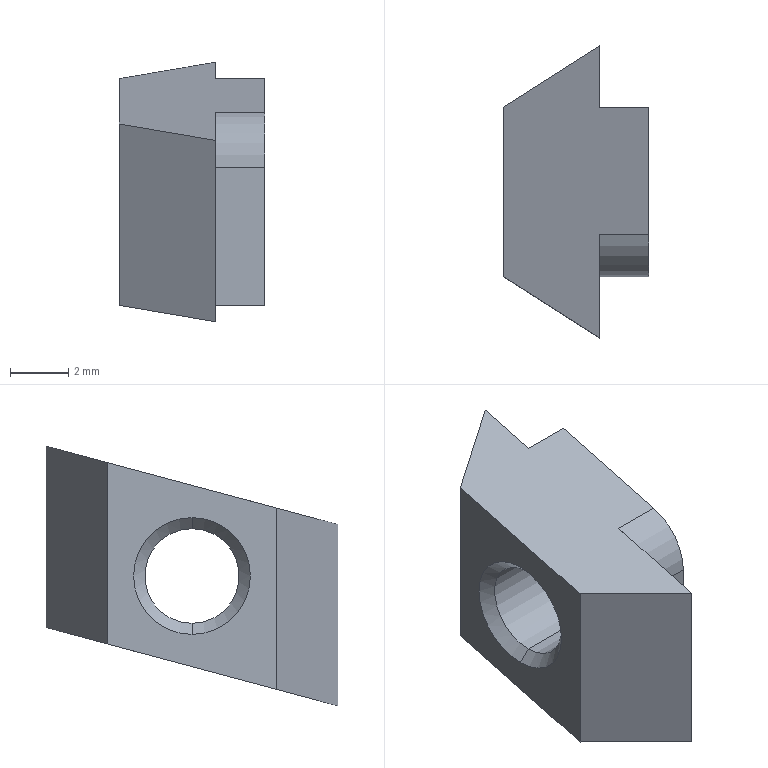Part | STEP file | 0245_026_HNTFSN5-4 | 1 solid | 18 faces | box 5 x 10 x 8.891 mm | volume 178.899 mm3 | plane 10 | cone 4 | cylinder 4 | commonest cylinder face diameters 3.242 x2 3.867 x2
STEP:
#1=CARTESIAN_POINT('',(0.,0.,0.));
#2=DIRECTION('',(0.,0.,1.));
#3=DIRECTION('',(1.,0.,0.));
#4=AXIS2_PLACEMENT_3D('',#1,#2,#3);
#5=CARTESIAN_POINT('',(-4.621,0.,1.621));
#6=VERTEX_POINT('',#5);
#7=CARTESIAN_POINT('',(-5.,0.,2.));
#8=VERTEX_POINT('',#7);
#9=CARTESIAN_POINT('',(-5.,0.,2.));
#10=DIRECTION('',(-0.7071,0.,0.7071));
#11=VECTOR('',#10,1.);
#12=LINE('',#9,#11);
#13=CARTESIAN_POINT('',(-5.,0.,0.));
#14=DIRECTION('',(-1.,0.,0.));
#15=DIRECTION('',(0.,0.,1.));
#16=AXIS2_PLACEMENT_3D('',#13,#14,#15);
#17=CONICAL_SURFACE('',#16,2.,0.7854);
#18=CARTESIAN_POINT('',(6.283,0.));
#19=DIRECTION('',(0.,1.));
#20=VECTOR('',#19,1.);
#21=LINE('',#18,#20);
#22=(GEOMETRIC_REPRESENTATION_CONTEXT(2)PARAMETRIC_REPRESENTATION_CONTEXT()REPRESENTATION_CONTEXT('',''));
#23=DEFINITIONAL_REPRESENTATION('',(#21),#22);
#24=PCURVE('',#17,#23);
#25=CARTESIAN_POINT('',(-5.,0.,0.));
#26=DIRECTION('',(-1.,0.,0.));
#27=DIRECTION('',(0.,0.,1.));
#28=AXIS2_PLACEMENT_3D('',#25,#26,#27);
#29=CONICAL_SURFACE('',#28,2.,0.7854);
#30=CARTESIAN_POINT('',(0.,0.));
#31=DIRECTION('',(0.,1.));
#32=VECTOR('',#31,1.);
#33=LINE('',#30,#32);
#34=(GEOMETRIC_REPRESENTATION_CONTEXT(2)PARAMETRIC_REPRESENTATION_CONTEXT()REPRESENTATION_CONTEXT('',''));
#35=DEFINITIONAL_REPRESENTATION('',(#33),#34);
#36=PCURVE('',#29,#35);
#37=SURFACE_CURVE('',#12,(#24,#36),.PCURVE_S1.);
#38=EDGE_CURVE('',#6,#8,#37,.T.);
#39=ORIENTED_EDGE('',*,*,#38,.T.);
#40=CARTESIAN_POINT('',(-5.,0.,-2.));
#41=VERTEX_POINT('',#40);
#42=CARTESIAN_POINT('',(-5.,0.,0.));
#43=DIRECTION('',(-1.,0.,0.));
#44=DIRECTION('',(0.,0.,1.));
#45=AXIS2_PLACEMENT_3D('',#42,#43,#44);
#46=CIRCLE('',#45,2.);
#47=CARTESIAN_POINT('',(0.,0.));
#48=DIRECTION('',(1.,0.));
#49=VECTOR('',#48,1.);
#50=LINE('',#47,#49);
#51=(GEOMETRIC_REPRESENTATION_CONTEXT(2)PARAMETRIC_REPRESENTATION_CONTEXT()REPRESENTATION_CONTEXT('',''));
#52=DEFINITIONAL_REPRESENTATION('',(#50),#51);
#53=PCURVE('',#17,#52);
#54=CARTESIAN_POINT('',(-5.,0.,0.));
#55=DIRECTION('',(1.,0.,0.));
#56=DIRECTION('',(0.,0.,-1.));
#57=AXIS2_PLACEMENT_3D('',#54,#55,#56);
#58=PLANE('',#57);
#59=CARTESIAN_POINT('',(-2.,0.));
#60=CARTESIAN_POINT('',(-2.,3.464));
#61=CARTESIAN_POINT('',(1.,1.732));
#62=CARTESIAN_POINT('',(4.,0.));
#63=CARTESIAN_POINT('',(1.,-1.732));
#64=CARTESIAN_POINT('',(-2.,-3.464));
#65=CARTESIAN_POINT('',(-2.,0.));
#66=(BOUNDED_CURVE()B_SPLINE_CURVE(2,(#59,#60,#61,#62,#63,#64,#65),.UNSPECIFIED.,.T.,.F.)B_SPLINE_CURVE_WITH_KNOTS((1,2,2,2,2,1),(-2.094,0.,2.094,4.189,6.283,8.378),.UNSPECIFIED.)CURVE()GEOMETRIC_REPRESENTATION_ITEM()RATIONAL_B_SPLINE_CURVE((1.,0.5,1.,0.5,1.,0.5,1.))REPRESENTATION_ITEM(''));
#67=(GEOMETRIC_REPRESENTATION_CONTEXT(2)PARAMETRIC_REPRESENTATION_CONTEXT()REPRESENTATION_CONTEXT('',''));
#68=DEFINITIONAL_REPRESENTATION('',(#66),#67);
#69=PCURVE('',#58,#68);
#70=SURFACE_CURVE('',#46,(#53,#69),.PCURVE_S1.);
#71=EDGE_CURVE('',#41,#8,#70,.T.);
#72=ORIENTED_EDGE('',*,*,#71,.F.);
#73=CARTESIAN_POINT('',(-4.621,0.,-1.621));
#74=VERTEX_POINT('',#73);
#75=CARTESIAN_POINT('',(-5.,0.,-2.));
#76=DIRECTION('',(-0.7071,0.,-0.7071));
#77=VECTOR('',#76,1.);
#78=LINE('',#75,#77);
#79=CARTESIAN_POINT('',(3.142,0.));
#80=DIRECTION('',(0.,1.));
#81=VECTOR('',#80,1.);
#82=LINE('',#79,#81);
#83=(GEOMETRIC_REPRESENTATION_CONTEXT(2)PARAMETRIC_REPRESENTATION_CONTEXT()REPRESENTATION_CONTEXT('',''));
#84=DEFINITIONAL_REPRESENTATION('',(#82),#83);
#85=PCURVE('',#17,#84);
#86=CARTESIAN_POINT('',(3.142,0.));
#87=DIRECTION('',(0.,1.));
#88=VECTOR('',#87,1.);
#89=LINE('',#86,#88);
#90=(GEOMETRIC_REPRESENTATION_CONTEXT(2)PARAMETRIC_REPRESENTATION_CONTEXT()REPRESENTATION_CONTEXT('',''));
#91=DEFINITIONAL_REPRESENTATION('',(#89),#90);
#92=PCURVE('',#29,#91);
#93=SURFACE_CURVE('',#78,(#85,#92),.PCURVE_S1.);
#94=EDGE_CURVE('',#74,#41,#93,.T.);
#95=ORIENTED_EDGE('',*,*,#94,.F.);
#96=CARTESIAN_POINT('',(-4.621,0.,0.));
#97=DIRECTION('',(-1.,0.,0.));
#98=DIRECTION('',(0.,1.,0.));
#99=AXIS2_PLACEMENT_3D('',#96,#97,#98);
#100=CIRCLE('',#99,1.621);
#101=CARTESIAN_POINT('',(1.571,-0.379));
#102=DIRECTION('',(1.,0.));
#103=VECTOR('',#102,1.);
#104=LINE('',#101,#103);
#105=(GEOMETRIC_REPRESENTATION_CONTEXT(2)PARAMETRIC_REPRESENTATION_CONTEXT()REPRESENTATION_CONTEXT('',''));
#106=DEFINITIONAL_REPRESENTATION('',(#104),#105);
#107=PCURVE('',#17,#106);
#108=CARTESIAN_POINT('',(-2.5,0.,0.));
#109=DIRECTION('',(1.,0.,0.));
#110=DIRECTION('',(0.,0.,-1.));
#111=AXIS2_PLACEMENT_3D('',#108,#109,#110);
#112=CYLINDRICAL_SURFACE('',#111,1.621);
#113=CARTESIAN_POINT('',(7.854,-2.121));
#114=DIRECTION('',(-1.,0.));
#115=VECTOR('',#114,1.);
#116=LINE('',#113,#115);
#117=(GEOMETRIC_REPRESENTATION_CONTEXT(2)PARAMETRIC_REPRESENTATION_CONTEXT()REPRESENTATION_CONTEXT('',''));
#118=DEFINITIONAL_REPRESENTATION('',(#116),#117);
#119=PCURVE('',#112,#118);
#120=SURFACE_CURVE('',#100,(#107,#119),.PCURVE_S1.);
#121=EDGE_CURVE('',#74,#6,#120,.T.);
#122=ORIENTED_EDGE('',*,*,#121,.T.);
#123=EDGE_LOOP('',(#39,#72,#95,#122));
#124=FACE_BOUND('',#123,.F.);
#125=ADVANCED_FACE('',(#124),#17,.F.);
#126=CARTESIAN_POINT('',(-0.379,0.,-1.621));
#127=VERTEX_POINT('',#126);
#128=CARTESIAN_POINT('',(0.,0.,-2.));
#129=VERTEX_POINT('',#128);
#130=CARTESIAN_POINT('',(0.,0.,-2.));
#131=DIRECTION('',(0.7071,0.,-0.7071));
#132=VECTOR('',#131,1.);
#133=LINE('',#130,#132);
#134=CARTESIAN_POINT('',(0.,0.,0.));
#135=DIRECTION('',(1.,0.,0.));
#136=DIRECTION('',(0.,0.,-1.));
#137=AXIS2_PLACEMENT_3D('',#134,#135,#136);
#138=CONICAL_SURFACE('',#137,2.,0.7854);
#139=CARTESIAN_POINT('',(6.283,0.));
#140=DIRECTION('',(0.,1.));
#141=VECTOR('',#140,1.);
#142=LINE('',#139,#141);
#143=(GEOMETRIC_REPRESENTATION_CONTEXT(2)PARAMETRIC_REPRESENTATION_CONTEXT()REPRESENTATION_CONTEXT('',''));
#144=DEFINITIONAL_REPRESENTATION('',(#142),#143);
#145=PCURVE('',#138,#144);
#146=CARTESIAN_POINT('',(0.,0.,0.));
#147=DIRECTION('',(1.,0.,0.));
#148=DIRECTION('',(0.,0.,-1.));
#149=AXIS2_PLACEMENT_3D('',#146,#147,#148);
#150=CONICAL_SURFACE('',#149,2.,0.7854);
#151=CARTESIAN_POINT('',(0.,0.));
#152=DIRECTION('',(0.,1.));
#153=VECTOR('',#152,1.);
#154=LINE('',#151,#153);
#155=(GEOMETRIC_REPRESENTATION_CONTEXT(2)PARAMETRIC_REPRESENTATION_CONTEXT()REPRESENTATION_CONTEXT('',''));
#156=DEFINITIONAL_REPRESENTATION('',(#154),#155);
#157=PCURVE('',#150,#156);
#158=SURFACE_CURVE('',#133,(#145,#157),.PCURVE_S1.);
#159=EDGE_CURVE('',#127,#129,#158,.T.);
#160=ORIENTED_EDGE('',*,*,#159,.T.);
#161=CARTESIAN_POINT('',(0.,0.,2.));
#162=VERTEX_POINT('',#161);
#163=CARTESIAN_POINT('',(0.,0.,0.));
#164=DIRECTION('',(-1.,0.,0.));
#165=DIRECTION('',(0.,0.,-1.));
#166=AXIS2_PLACEMENT_3D('',#163,#164,#165);
#167=CIRCLE('',#166,2.);
#168=CARTESIAN_POINT('',(6.283,0.));
#169=DIRECTION('',(-1.,0.));
#170=VECTOR('',#169,1.);
#171=LINE('',#168,#170);
#172=(GEOMETRIC_REPRESENTATION_CONTEXT(2)PARAMETRIC_REPRESENTATION_CONTEXT()REPRESENTATION_CONTEXT('',''));
#173=DEFINITIONAL_REPRESENTATION('',(#171),#172);
#174=PCURVE('',#138,#173);
#175=CARTESIAN_POINT('',(0.,0.,0.));
#176=DIRECTION('',(1.,0.,0.));
#177=DIRECTION('',(0.,0.,-1.));
#178=AXIS2_PLACEMENT_3D('',#175,#176,#177);
#179=PLANE('',#178);
#180=CARTESIAN_POINT('',(2.,0.));
#181=CARTESIAN_POINT('',(2.,-3.464));
#182=CARTESIAN_POINT('',(-1.,-1.732));
#183=CARTESIAN_POINT('',(-4.,0.));
#184=CARTESIAN_POINT('',(-1.,1.732));
#185=CARTESIAN_POINT('',(2.,3.464));
#186=CARTESIAN_POINT('',(2.,0.));
#187=(BOUNDED_CURVE()B_SPLINE_CURVE(2,(#180,#181,#182,#183,#184,#185,#186),.UNSPECIFIED.,.T.,.F.)B_SPLINE_CURVE_WITH_KNOTS((1,2,2,2,2,1),(-2.094,0.,2.094,4.189,6.283,8.378),.UNSPECIFIED.)CURVE()GEOMETRIC_REPRESENTATION_ITEM()RATIONAL_B_SPLINE_CURVE((1.,0.5,1.,0.5,1.,0.5,1.))REPRESENTATION_ITEM(''));
#188=(GEOMETRIC_REPRESENTATION_CONTEXT(2)PARAMETRIC_REPRESENTATION_CONTEXT()REPRESENTATION_CONTEXT('',''));
#189=DEFINITIONAL_REPRESENTATION('',(#187),#188);
#190=PCURVE('',#179,#189);
#191=SURFACE_CURVE('',#167,(#174,#190),.PCURVE_S1.);
#192=EDGE_CURVE('',#129,#162,#191,.T.);
#193=ORIENTED_EDGE('',*,*,#192,.T.);
#194=CARTESIAN_POINT('',(-0.379,0.,1.621));
#195=VERTEX_POINT('',#194);
#196=CARTESIAN_POINT('',(0.,0.,2.));
#197=DIRECTION('',(0.7071,0.,0.7071));
#198=VECTOR('',#197,1.);
#199=LINE('',#196,#198);
#200=CARTESIAN_POINT('',(3.142,0.));
#201=DIRECTION('',(0.,1.));
#202=VECTOR('',#201,1.);
#203=LINE('',#200,#202);
#204=(GEOMETRIC_REPRESENTATION_CONTEXT(2)PARAMETRIC_REPRESENTATION_CONTEXT()REPRESENTATION_CONTEXT('',''));
#205=DEFINITIONAL_REPRESENTATION('',(#203),#204);
#206=PCURVE('',#138,#205);
#207=CARTESIAN_POINT('',(3.142,0.));
#208=DIRECTION('',(0.,1.));
#209=VECTOR('',#208,1.);
#210=LINE('',#207,#209);
#211=(GEOMETRIC_REPRESENTATION_CONTEXT(2)PARAMETRIC_REPRESENTATION_CONTEXT()REPRESENTATION_CONTEXT('',''));
#212=DEFINITIONAL_REPRESENTATION('',(#210),#211);
#213=PCURVE('',#150,#212);
#214=SURFACE_CURVE('',#199,(#206,#213),.PCURVE_S1.);
#215=EDGE_CURVE('',#195,#162,#214,.T.);
#216=ORIENTED_EDGE('',*,*,#215,.F.);
#217=CARTESIAN_POINT('',(-0.379,0.,0.));
#218=DIRECTION('',(1.,0.,0.));
#219=DIRECTION('',(0.,1.,0.));
#220=AXIS2_PLACEMENT_3D('',#217,#218,#219);
#221=CIRCLE('',#220,1.621);
#222=CARTESIAN_POINT('',(1.571,-0.379));
#223=DIRECTION('',(1.,0.));
#224=VECTOR('',#223,1.);
#225=LINE('',#222,#224);
#226=(GEOMETRIC_REPRESENTATION_CONTEXT(2)PARAMETRIC_REPRESENTATION_CONTEXT()REPRESENTATION_CONTEXT('',''));
#227=DEFINITIONAL_REPRESENTATION('',(#225),#226);
#228=PCURVE('',#138,#227);
#229=CARTESIAN_POINT('',(1.571,2.121));
#230=DIRECTION('',(1.,0.));
#231=VECTOR('',#230,1.);
#232=LINE('',#229,#231);
#233=(GEOMETRIC_REPRESENTATION_CONTEXT(2)PARAMETRIC_REPRESENTATION_CONTEXT()REPRESENTATION_CONTEXT('',''));
#234=DEFINITIONAL_REPRESENTATION('',(#232),#233);
#235=PCURVE('',#112,#234);
#236=SURFACE_CURVE('',#221,(#228,#235),.PCURVE_S1.);
#237=EDGE_CURVE('',#195,#127,#236,.T.);
#238=ORIENTED_EDGE('',*,*,#237,.T.);
#239=EDGE_LOOP('',(#160,#193,#216,#238));
#240=FACE_BOUND('',#239,.F.);
#241=ADVANCED_FACE('',(#240),#138,.F.);
#242=CARTESIAN_POINT('',(-2.5,0.,-1.621));
#243=DIRECTION('',(1.,0.,0.));
#244=VECTOR('',#243,1.);
#245=LINE('',#242,#244);
#246=CARTESIAN_POINT('',(6.283,0.));
#247=DIRECTION('',(0.,1.));
#248=VECTOR('',#247,1.);
#249=LINE('',#246,#248);
#250=(GEOMETRIC_REPRESENTATION_CONTEXT(2)PARAMETRIC_REPRESENTATION_CONTEXT()REPRESENTATION_CONTEXT('',''));
#251=DEFINITIONAL_REPRESENTATION('',(#249),#250);
#252=PCURVE('',#112,#251);
#253=CARTESIAN_POINT('',(-2.5,0.,0.));
#254=DIRECTION('',(1.,0.,0.));
#255=DIRECTION('',(0.,0.,-1.));
#256=AXIS2_PLACEMENT_3D('',#253,#254,#255);
#257=CYLINDRICAL_SURFACE('',#256,1.621);
#258=CARTESIAN_POINT('',(0.,0.));
#259=DIRECTION('',(0.,1.));
#260=VECTOR('',#259,1.);
#261=LINE('',#258,#260);
#262=(GEOMETRIC_REPRESENTATION_CONTEXT(2)PARAMETRIC_REPRESENTATION_CONTEXT()REPRESENTATION_CONTEXT('',''));
#263=DEFINITIONAL_REPRESENTATION('',(#261),#262);
#264=PCURVE('',#257,#263);
#265=SURFACE_CURVE('',#245,(#252,#264),.PCURVE_S1.);
#266=EDGE_CURVE('',#74,#127,#265,.T.);
#267=ORIENTED_EDGE('',*,*,#266,.T.);
#268=ORIENTED_EDGE('',*,*,#237,.F.);
#269=CARTESIAN_POINT('',(-2.5,0.,1.621));
#270=DIRECTION('',(1.,0.,0.));
#271=VECTOR('',#270,1.);
#272=LINE('',#269,#271);
#273=CARTESIAN_POINT('',(3.142,0.));
#274=DIRECTION('',(0.,1.));
#275=VECTOR('',#274,1.);
#276=LINE('',#273,#275);
#277=(GEOMETRIC_REPRESENTATION_CONTEXT(2)PARAMETRIC_REPRESENTATION_CONTEXT()REPRESENTATION_CONTEXT('',''));
#278=DEFINITIONAL_REPRESENTATION('',(#276),#277);
#279=PCURVE('',#112,#278);
#280=CARTESIAN_POINT('',(3.142,0.));
#281=DIRECTION('',(0.,1.));
#282=VECTOR('',#281,1.);
#283=LINE('',#280,#282);
#284=(GEOMETRIC_REPRESENTATION_CONTEXT(2)PARAMETRIC_REPRESENTATION_CONTEXT()REPRESENTATION_CONTEXT('',''));
#285=DEFINITIONAL_REPRESENTATION('',(#283),#284);
#286=PCURVE('',#257,#285);
#287=SURFACE_CURVE('',#272,(#279,#286),.PCURVE_S1.);
#288=EDGE_CURVE('',#6,#195,#287,.T.);
#289=ORIENTED_EDGE('',*,*,#288,.F.);
#290=ORIENTED_EDGE('',*,*,#121,.F.);
#291=EDGE_LOOP('',(#267,#268,#289,#290));
#292=FACE_BOUND('',#291,.F.);
#293=ADVANCED_FACE('',(#292),#112,.F.);
#294=CARTESIAN_POINT('',(-5.,-2.9,-3.883));
#295=VERTEX_POINT('',#294);
#296=CARTESIAN_POINT('',(-5.,2.9,-2.329));
#297=VERTEX_POINT('',#296);
#298=CARTESIAN_POINT('',(-5.,-5.,-4.446));
#299=DIRECTION('',(0.,0.9659,0.2588));
#300=VECTOR('',#299,1.);
#301=LINE('',#298,#300);
#302=CARTESIAN_POINT('',(0.,-5.,-4.446));
#303=DIRECTION('',(0.,0.2588,-0.9659));
#304=DIRECTION('',(0.,0.9659,0.2588));
#305=AXIS2_PLACEMENT_3D('',#302,#303,#304);
#306=PLANE('',#305);
#307=CARTESIAN_POINT('',(0.,-5.));
#308=DIRECTION('',(1.,0.));
#309=VECTOR('',#308,1.);
#310=LINE('',#307,#309);
#311=(GEOMETRIC_REPRESENTATION_CONTEXT(2)PARAMETRIC_REPRESENTATION_CONTEXT()REPRESENTATION_CONTEXT('',''));
#312=DEFINITIONAL_REPRESENTATION('',(#310),#311);
#313=PCURVE('',#306,#312);
#314=CARTESIAN_POINT('',(4.446,-5.));
#315=DIRECTION('',(-0.2588,0.9659));
#316=VECTOR('',#315,1.);
#317=LINE('',#314,#316);
#318=(GEOMETRIC_REPRESENTATION_CONTEXT(2)PARAMETRIC_REPRESENTATION_CONTEXT()REPRESENTATION_CONTEXT('',''));
#319=DEFINITIONAL_REPRESENTATION('',(#317),#318);
#320=PCURVE('',#58,#319);
#321=SURFACE_CURVE('',#301,(#313,#320),.PCURVE_S1.);
#322=EDGE_CURVE('',#295,#297,#321,.T.);
#323=ORIENTED_EDGE('',*,*,#322,.T.);
#324=CARTESIAN_POINT('',(-1.7,5.,-1.766));
#325=VERTEX_POINT('',#324);
#326=CARTESIAN_POINT('',(-5.,2.9,-2.329));
#327=DIRECTION('',(0.8351,0.5314,0.1424));
#328=VECTOR('',#327,1.);
#329=LINE('',#326,#328);
#330=CARTESIAN_POINT('',(8.179,-5.));
#331=DIRECTION('',(0.5502,0.8351));
#332=VECTOR('',#331,1.);
#333=LINE('',#330,#332);
#334=(GEOMETRIC_REPRESENTATION_CONTEXT(2)PARAMETRIC_REPRESENTATION_CONTEXT()REPRESENTATION_CONTEXT('',''));
#335=DEFINITIONAL_REPRESENTATION('',(#333),#334);
#336=PCURVE('',#306,#335);
#337=CARTESIAN_POINT('',(-5.,2.9,12.));
#338=DIRECTION('',(0.5369,-0.8437,0.));
#339=DIRECTION('',(0.8437,0.5369,0.));
#340=AXIS2_PLACEMENT_3D('',#337,#338,#339);
#341=PLANE('',#340);
#342=CARTESIAN_POINT('',(0.,-14.329));
#343=DIRECTION('',(0.9898,0.1424));
#344=VECTOR('',#343,1.);
#345=LINE('',#342,#344);
#346=(GEOMETRIC_REPRESENTATION_CONTEXT(2)PARAMETRIC_REPRESENTATION_CONTEXT()REPRESENTATION_CONTEXT('',''));
#347=DEFINITIONAL_REPRESENTATION('',(#345),#346);
#348=PCURVE('',#341,#347);
#349=SURFACE_CURVE('',#329,(#336,#348),.PCURVE_S1.);
#350=EDGE_CURVE('',#297,#325,#349,.T.);
#351=ORIENTED_EDGE('',*,*,#350,.T.);
#352=CARTESIAN_POINT('',(-1.7,1.467,-2.713));
#353=VERTEX_POINT('',#352);
#354=CARTESIAN_POINT('',(-1.7,-5.,-4.446));
#355=DIRECTION('',(0.,-0.9659,-0.2588));
#356=VECTOR('',#355,1.);
#357=LINE('',#354,#356);
#358=CARTESIAN_POINT('',(0.,-1.7));
#359=DIRECTION('',(-1.,0.));
#360=VECTOR('',#359,1.);
#361=LINE('',#358,#360);
#362=(GEOMETRIC_REPRESENTATION_CONTEXT(2)PARAMETRIC_REPRESENTATION_CONTEXT()REPRESENTATION_CONTEXT('',''));
#363=DEFINITIONAL_REPRESENTATION('',(#361),#362);
#364=PCURVE('',#306,#363);
#365=CARTESIAN_POINT('',(-1.7,5.,12.));
#366=DIRECTION('',(-1.,0.,0.));
#367=DIRECTION('',(0.,0.,1.));
#368=AXIS2_PLACEMENT_3D('',#365,#366,#367);
#369=PLANE('',#368);
#370=CARTESIAN_POINT('',(-16.446,-10.));
#371=DIRECTION('',(-0.2588,-0.9659));
#372=VECTOR('',#371,1.);
#373=LINE('',#370,#372);
#374=(GEOMETRIC_REPRESENTATION_CONTEXT(2)PARAMETRIC_REPRESENTATION_CONTEXT()REPRESENTATION_CONTEXT('',''));
#375=DEFINITIONAL_REPRESENTATION('',(#373),#374);
#376=PCURVE('',#369,#375);
#377=SURFACE_CURVE('',#357,(#364,#376),.PCURVE_S1.);
#378=EDGE_CURVE('',#325,#353,#377,.T.);
#379=ORIENTED_EDGE('',*,*,#378,.T.);
#380=CARTESIAN_POINT('',(0.,1.467,-2.713));
#381=VERTEX_POINT('',#380);
#382=CARTESIAN_POINT('',(-1.7,1.467,-2.713));
#383=DIRECTION('',(-1.,0.,0.));
#384=VECTOR('',#383,1.);
#385=LINE('',#382,#384);
#386=CARTESIAN_POINT('',(6.695,-1.7));
#387=DIRECTION('',(0.,-1.));
#388=VECTOR('',#387,1.);
#389=LINE('',#386,#388);
#390=(GEOMETRIC_REPRESENTATION_CONTEXT(2)PARAMETRIC_REPRESENTATION_CONTEXT()REPRESENTATION_CONTEXT('',''));
#391=DEFINITIONAL_REPRESENTATION('',(#389),#390);
#392=PCURVE('',#306,#391);
#393=CARTESIAN_POINT('',(-1.7,0.9667,-0.8453));
#394=DIRECTION('',(-1.,0.,0.));
#395=DIRECTION('',(0.,0.,1.));
#396=AXIS2_PLACEMENT_3D('',#393,#394,#395);
#397=CYLINDRICAL_SURFACE('',#396,1.933);
#398=CARTESIAN_POINT('',(2.88,0.));
#399=DIRECTION('',(0.,1.));
#400=VECTOR('',#399,1.);
#401=LINE('',#398,#400);
#402=(GEOMETRIC_REPRESENTATION_CONTEXT(2)PARAMETRIC_REPRESENTATION_CONTEXT()REPRESENTATION_CONTEXT('',''));
#403=DEFINITIONAL_REPRESENTATION('',(#401),#402);
#404=PCURVE('',#397,#403);
#405=SURFACE_CURVE('',#385,(#392,#404),.PCURVE_S1.);
#406=EDGE_CURVE('',#381,#353,#405,.T.);
#407=ORIENTED_EDGE('',*,*,#406,.F.);
#408=CARTESIAN_POINT('',(0.,-2.9,-3.883));
#409=VERTEX_POINT('',#408);
#410=CARTESIAN_POINT('',(0.,-5.,-4.446));
#411=DIRECTION('',(0.,-0.9659,-0.2588));
#412=VECTOR('',#411,1.);
#413=LINE('',#410,#412);
#414=CARTESIAN_POINT('',(0.,0.));
#415=DIRECTION('',(-1.,0.));
#416=VECTOR('',#415,1.);
#417=LINE('',#414,#416);
#418=(GEOMETRIC_REPRESENTATION_CONTEXT(2)PARAMETRIC_REPRESENTATION_CONTEXT()REPRESENTATION_CONTEXT('',''));
#419=DEFINITIONAL_REPRESENTATION('',(#417),#418);
#420=PCURVE('',#306,#419);
#421=CARTESIAN_POINT('',(4.446,-5.));
#422=DIRECTION('',(0.2588,-0.9659));
#423=VECTOR('',#422,1.);
#424=LINE('',#421,#423);
#425=(GEOMETRIC_REPRESENTATION_CONTEXT(2)PARAMETRIC_REPRESENTATION_CONTEXT()REPRESENTATION_CONTEXT('',''));
#426=DEFINITIONAL_REPRESENTATION('',(#424),#425);
#427=PCURVE('',#179,#426);
#428=SURFACE_CURVE('',#413,(#420,#427),.PCURVE_S1.);
#429=EDGE_CURVE('',#381,#409,#428,.T.);
#430=ORIENTED_EDGE('',*,*,#429,.T.);
#431=CARTESIAN_POINT('',(-1.7,-2.9,-3.883));
#432=VERTEX_POINT('',#431);
#433=CARTESIAN_POINT('',(0.,-2.9,-3.883));
#434=DIRECTION('',(-1.,0.,0.));
#435=VECTOR('',#434,1.);
#436=LINE('',#433,#435);
#437=CARTESIAN_POINT('',(2.174,0.));
#438=DIRECTION('',(0.,-1.));
#439=VECTOR('',#438,1.);
#440=LINE('',#437,#439);
#441=(GEOMETRIC_REPRESENTATION_CONTEXT(2)PARAMETRIC_REPRESENTATION_CONTEXT()REPRESENTATION_CONTEXT('',''));
#442=DEFINITIONAL_REPRESENTATION('',(#440),#441);
#443=PCURVE('',#306,#442);
#444=CARTESIAN_POINT('',(0.,-2.9,12.));
#445=DIRECTION('',(0.,1.,0.));
#446=DIRECTION('',(-1.,0.,0.));
#447=AXIS2_PLACEMENT_3D('',#444,#445,#446);
#448=PLANE('',#447);
#449=CARTESIAN_POINT('',(0.,-15.883));
#450=DIRECTION('',(1.,0.));
#451=VECTOR('',#450,1.);
#452=LINE('',#449,#451);
#453=(GEOMETRIC_REPRESENTATION_CONTEXT(2)PARAMETRIC_REPRESENTATION_CONTEXT()REPRESENTATION_CONTEXT('',''));
#454=DEFINITIONAL_REPRESENTATION('',(#452),#453);
#455=PCURVE('',#448,#454);
#456=SURFACE_CURVE('',#436,(#443,#455),.PCURVE_S1.);
#457=EDGE_CURVE('',#409,#432,#456,.T.);
#458=ORIENTED_EDGE('',*,*,#457,.T.);
#459=CARTESIAN_POINT('',(-1.7,-5.,-4.446));
#460=VERTEX_POINT('',#459);
#461=CARTESIAN_POINT('',(-1.7,-5.,-4.446));
#462=DIRECTION('',(0.,-0.9659,-0.2588));
#463=VECTOR('',#462,1.);
#464=LINE('',#461,#463);
#465=CARTESIAN_POINT('',(0.,-1.7));
#466=DIRECTION('',(-1.,0.));
#467=VECTOR('',#466,1.);
#468=LINE('',#465,#467);
#469=(GEOMETRIC_REPRESENTATION_CONTEXT(2)PARAMETRIC_REPRESENTATION_CONTEXT()REPRESENTATION_CONTEXT('',''));
#470=DEFINITIONAL_REPRESENTATION('',(#468),#469);
#471=PCURVE('',#306,#470);
#472=CARTESIAN_POINT('',(-1.7,-2.9,12.));
#473=DIRECTION('',(-1.,0.,0.));
#474=DIRECTION('',(0.,0.,1.));
#475=AXIS2_PLACEMENT_3D('',#472,#473,#474);
#476=PLANE('',#475);
#477=CARTESIAN_POINT('',(-16.446,-2.1));
#478=DIRECTION('',(-0.2588,-0.9659));
#479=VECTOR('',#478,1.);
#480=LINE('',#477,#479);
#481=(GEOMETRIC_REPRESENTATION_CONTEXT(2)PARAMETRIC_REPRESENTATION_CONTEXT()REPRESENTATION_CONTEXT('',''));
#482=DEFINITIONAL_REPRESENTATION('',(#480),#481);
#483=PCURVE('',#476,#482);
#484=SURFACE_CURVE('',#464,(#471,#483),.PCURVE_S1.);
#485=EDGE_CURVE('',#432,#460,#484,.T.);
#486=ORIENTED_EDGE('',*,*,#485,.T.);
#487=CARTESIAN_POINT('',(-1.7,-5.,-4.446));
#488=DIRECTION('',(-0.8351,0.5314,0.1424));
#489=VECTOR('',#488,1.);
#490=LINE('',#487,#489);
#491=CARTESIAN_POINT('',(0.,-1.7));
#492=DIRECTION('',(0.5502,-0.8351));
#493=VECTOR('',#492,1.);
#494=LINE('',#491,#493);
#495=(GEOMETRIC_REPRESENTATION_CONTEXT(2)PARAMETRIC_REPRESENTATION_CONTEXT()REPRESENTATION_CONTEXT('',''));
#496=DEFINITIONAL_REPRESENTATION('',(#494),#495);
#497=PCURVE('',#306,#496);
#498=CARTESIAN_POINT('',(-1.7,-5.,12.));
#499=DIRECTION('',(0.5369,0.8437,0.));
#500=DIRECTION('',(-0.8437,0.5369,0.));
#501=AXIS2_PLACEMENT_3D('',#498,#499,#500);
#502=PLANE('',#501);
#503=CARTESIAN_POINT('',(0.,-16.446));
#504=DIRECTION('',(0.9898,0.1424));
#505=VECTOR('',#504,1.);
#506=LINE('',#503,#505);
#507=(GEOMETRIC_REPRESENTATION_CONTEXT(2)PARAMETRIC_REPRESENTATION_CONTEXT()REPRESENTATION_CONTEXT('',''));
#508=DEFINITIONAL_REPRESENTATION('',(#506),#507);
#509=PCURVE('',#502,#508);
#510=SURFACE_CURVE('',#490,(#497,#509),.PCURVE_S1.);
#511=EDGE_CURVE('',#460,#295,#510,.T.);
#512=ORIENTED_EDGE('',*,*,#511,.T.);
#513=EDGE_LOOP('',(#323,#351,#379,#407,#430,#458,#486,#512));
#514=FACE_BOUND('',#513,.T.);
#515=ADVANCED_FACE('',(#514),#306,.T.);
#516=CARTESIAN_POINT('',(-5.,2.9,3.883));
#517=VERTEX_POINT('',#516);
#518=CARTESIAN_POINT('',(-5.,2.9,12.));
#519=DIRECTION('',(0.,0.,-1.));
#520=VECTOR('',#519,1.);
#521=LINE('',#518,#520);
#522=CARTESIAN_POINT('',(0.,0.));
#523=DIRECTION('',(0.,-1.));
#524=VECTOR('',#523,1.);
#525=LINE('',#522,#524);
#526=(GEOMETRIC_REPRESENTATION_CONTEXT(2)PARAMETRIC_REPRESENTATION_CONTEXT()REPRESENTATION_CONTEXT('',''));
#527=DEFINITIONAL_REPRESENTATION('',(#525),#526);
#528=PCURVE('',#341,#527);
#529=CARTESIAN_POINT('',(-12.,2.9));
#530=DIRECTION('',(1.,0.));
#531=VECTOR('',#530,1.);
#532=LINE('',#529,#531);
#533=(GEOMETRIC_REPRESENTATION_CONTEXT(2)PARAMETRIC_REPRESENTATION_CONTEXT()REPRESENTATION_CONTEXT('',''));
#534=DEFINITIONAL_REPRESENTATION('',(#532),#533);
#535=PCURVE('',#58,#534);
#536=SURFACE_CURVE('',#521,(#528,#535),.PCURVE_S1.);
#537=EDGE_CURVE('',#517,#297,#536,.T.);
#538=ORIENTED_EDGE('',*,*,#537,.F.);
#539=CARTESIAN_POINT('',(-1.7,5.,4.446));
#540=VERTEX_POINT('',#539);
#541=CARTESIAN_POINT('',(-1.7,5.,4.446));
#542=DIRECTION('',(-0.8351,-0.5314,-0.1424));
#543=VECTOR('',#542,1.);
#544=LINE('',#541,#543);
#545=CARTESIAN_POINT('',(3.912,-7.554));
#546=DIRECTION('',(-0.9898,-0.1424));
#547=VECTOR('',#546,1.);
#548=LINE('',#545,#547);
#549=(GEOMETRIC_REPRESENTATION_CONTEXT(2)PARAMETRIC_REPRESENTATION_CONTEXT()REPRESENTATION_CONTEXT('',''));
#550=DEFINITIONAL_REPRESENTATION('',(#548),#549);
#551=PCURVE('',#341,#550);
#552=CARTESIAN_POINT('',(0.,5.,4.446));
#553=DIRECTION('',(0.,-0.2588,0.9659));
#554=DIRECTION('',(0.,-0.9659,-0.2588));
#555=AXIS2_PLACEMENT_3D('',#552,#553,#554);
#556=PLANE('',#555);
#557=CARTESIAN_POINT('',(0.,-1.7));
#558=DIRECTION('',(0.5502,-0.8351));
#559=VECTOR('',#558,1.);
#560=LINE('',#557,#559);
#561=(GEOMETRIC_REPRESENTATION_CONTEXT(2)PARAMETRIC_REPRESENTATION_CONTEXT()REPRESENTATION_CONTEXT('',''));
#562=DEFINITIONAL_REPRESENTATION('',(#560),#561);
#563=PCURVE('',#556,#562);
#564=SURFACE_CURVE('',#544,(#551,#563),.PCURVE_S1.);
#565=EDGE_CURVE('',#540,#517,#564,.T.);
#566=ORIENTED_EDGE('',*,*,#565,.F.);
#567=CARTESIAN_POINT('',(-1.7,5.,12.));
#568=DIRECTION('',(0.,0.,1.));
#569=VECTOR('',#568,1.);
#570=LINE('',#567,#569);
#571=CARTESIAN_POINT('',(3.912,0.));
#572=DIRECTION('',(0.,1.));
#573=VECTOR('',#572,1.);
#574=LINE('',#571,#573);
#575=(GEOMETRIC_REPRESENTATION_CONTEXT(2)PARAMETRIC_REPRESENTATION_CONTEXT()REPRESENTATION_CONTEXT('',''));
#576=DEFINITIONAL_REPRESENTATION('',(#574),#575);
#577=PCURVE('',#341,#576);
#578=CARTESIAN_POINT('',(0.,0.));
#579=DIRECTION('',(1.,0.));
#580=VECTOR('',#579,1.);
#581=LINE('',#578,#580);
#582=(GEOMETRIC_REPRESENTATION_CONTEXT(2)PARAMETRIC_REPRESENTATION_CONTEXT()REPRESENTATION_CONTEXT('',''));
#583=DEFINITIONAL_REPRESENTATION('',(#581),#582);
#584=PCURVE('',#369,#583);
#585=SURFACE_CURVE('',#570,(#577,#584),.PCURVE_S1.);
#586=EDGE_CURVE('',#325,#540,#585,.T.);
#587=ORIENTED_EDGE('',*,*,#586,.F.);
#588=ORIENTED_EDGE('',*,*,#350,.F.);
#589=EDGE_LOOP('',(#538,#566,#587,#588));
#590=FACE_BOUND('',#589,.T.);
#591=ADVANCED_FACE('',(#590),#341,.F.);
#592=ORIENTED_EDGE('',*,*,#322,.F.);
#593=CARTESIAN_POINT('',(-5.,-2.9,2.329));
#594=VERTEX_POINT('',#593);
#595=CARTESIAN_POINT('',(-5.,-2.9,0.));
#596=DIRECTION('',(0.,0.,-1.));
#597=VECTOR('',#596,1.);
#598=LINE('',#595,#597);
#599=CARTESIAN_POINT('',(0.,-2.9));
#600=DIRECTION('',(1.,0.));
#601=VECTOR('',#600,1.);
#602=LINE('',#599,#601);
#603=(GEOMETRIC_REPRESENTATION_CONTEXT(2)PARAMETRIC_REPRESENTATION_CONTEXT()REPRESENTATION_CONTEXT('',''));
#604=DEFINITIONAL_REPRESENTATION('',(#602),#603);
#605=PCURVE('',#58,#604);
#606=CARTESIAN_POINT('',(3.912,-12.));
#607=DIRECTION('',(0.,-1.));
#608=VECTOR('',#607,1.);
#609=LINE('',#606,#608);
#610=(GEOMETRIC_REPRESENTATION_CONTEXT(2)PARAMETRIC_REPRESENTATION_CONTEXT()REPRESENTATION_CONTEXT('',''));
#611=DEFINITIONAL_REPRESENTATION('',(#609),#610);
#612=PCURVE('',#502,#611);
#613=SURFACE_CURVE('',#598,(#605,#612),.PCURVE_S1.);
#614=EDGE_CURVE('',#594,#295,#613,.T.);
#615=ORIENTED_EDGE('',*,*,#614,.F.);
#616=CARTESIAN_POINT('',(-5.,2.9,3.883));
#617=DIRECTION('',(0.,-0.9659,-0.2588));
#618=VECTOR('',#617,1.);
#619=LINE('',#616,#618);
#620=CARTESIAN_POINT('',(-3.883,2.9));
#621=DIRECTION('',(0.2588,-0.9659));
#622=VECTOR('',#621,1.);
#623=LINE('',#620,#622);
#624=(GEOMETRIC_REPRESENTATION_CONTEXT(2)PARAMETRIC_REPRESENTATION_CONTEXT()REPRESENTATION_CONTEXT('',''));
#625=DEFINITIONAL_REPRESENTATION('',(#623),#624);
#626=PCURVE('',#58,#625);
#627=CARTESIAN_POINT('',(2.174,-5.));
#628=DIRECTION('',(1.,0.));
#629=VECTOR('',#628,1.);
#630=LINE('',#627,#629);
#631=(GEOMETRIC_REPRESENTATION_CONTEXT(2)PARAMETRIC_REPRESENTATION_CONTEXT()REPRESENTATION_CONTEXT('',''));
#632=DEFINITIONAL_REPRESENTATION('',(#630),#631);
#633=PCURVE('',#556,#632);
#634=SURFACE_CURVE('',#619,(#626,#633),.PCURVE_S1.);
#635=EDGE_CURVE('',#517,#594,#634,.T.);
#636=ORIENTED_EDGE('',*,*,#635,.F.);
#637=ORIENTED_EDGE('',*,*,#537,.T.);
#638=EDGE_LOOP('',(#592,#615,#636,#637));
#639=FACE_BOUND('',#638,.T.);
#640=CARTESIAN_POINT('',(-5.,0.,0.));
#641=DIRECTION('',(-1.,0.,0.));
#642=DIRECTION('',(0.,0.,1.));
#643=AXIS2_PLACEMENT_3D('',#640,#641,#642);
#644=CIRCLE('',#643,2.);
#645=CARTESIAN_POINT('',(-2.,0.));
#646=CARTESIAN_POINT('',(-2.,3.464));
#647=CARTESIAN_POINT('',(1.,1.732));
#648=CARTESIAN_POINT('',(4.,0.));
#649=CARTESIAN_POINT('',(1.,-1.732));
#650=CARTESIAN_POINT('',(-2.,-3.464));
#651=CARTESIAN_POINT('',(-2.,0.));
#652=(BOUNDED_CURVE()B_SPLINE_CURVE(2,(#645,#646,#647,#648,#649,#650,#651),.UNSPECIFIED.,.T.,.F.)B_SPLINE_CURVE_WITH_KNOTS((1,2,2,2,2,1),(-2.094,0.,2.094,4.189,6.283,8.378),.UNSPECIFIED.)CURVE()GEOMETRIC_REPRESENTATION_ITEM()RATIONAL_B_SPLINE_CURVE((1.,0.5,1.,0.5,1.,0.5,1.))REPRESENTATION_ITEM(''));
#653=(GEOMETRIC_REPRESENTATION_CONTEXT(2)PARAMETRIC_REPRESENTATION_CONTEXT()REPRESENTATION_CONTEXT('',''));
#654=DEFINITIONAL_REPRESENTATION('',(#652),#653);
#655=PCURVE('',#58,#654);
#656=CARTESIAN_POINT('',(0.,0.));
#657=DIRECTION('',(1.,0.));
#658=VECTOR('',#657,1.);
#659=LINE('',#656,#658);
#660=(GEOMETRIC_REPRESENTATION_CONTEXT(2)PARAMETRIC_REPRESENTATION_CONTEXT()REPRESENTATION_CONTEXT('',''));
#661=DEFINITIONAL_REPRESENTATION('',(#659),#660);
#662=PCURVE('',#29,#661);
#663=SURFACE_CURVE('',#644,(#655,#662),.PCURVE_S1.);
#664=EDGE_CURVE('',#8,#41,#663,.T.);
#665=ORIENTED_EDGE('',*,*,#664,.F.);
#666=ORIENTED_EDGE('',*,*,#71,.F.);
#667=EDGE_LOOP('',(#665,#666));
#668=FACE_BOUND('',#667,.T.);
#669=ADVANCED_FACE('',(#639,#668),#58,.F.);
#670=CARTESIAN_POINT('',(-1.7,-5.,1.766));
#671=VERTEX_POINT('',#670);
#672=CARTESIAN_POINT('',(-1.7,-5.,12.));
#673=DIRECTION('',(0.,0.,-1.));
#674=VECTOR('',#673,1.);
#675=LINE('',#672,#674);
#676=CARTESIAN_POINT('',(0.,0.));
#677=DIRECTION('',(0.,-1.));
#678=VECTOR('',#677,1.);
#679=LINE('',#676,#678);
#680=(GEOMETRIC_REPRESENTATION_CONTEXT(2)PARAMETRIC_REPRESENTATION_CONTEXT()REPRESENTATION_CONTEXT('',''));
#681=DEFINITIONAL_REPRESENTATION('',(#679),#680);
#682=PCURVE('',#502,#681);
#683=CARTESIAN_POINT('',(0.,-2.1));
#684=DIRECTION('',(-1.,0.));
#685=VECTOR('',#684,1.);
#686=LINE('',#683,#685);
#687=(GEOMETRIC_REPRESENTATION_CONTEXT(2)PARAMETRIC_REPRESENTATION_CONTEXT()REPRESENTATION_CONTEXT('',''));
#688=DEFINITIONAL_REPRESENTATION('',(#686),#687);
#689=PCURVE('',#476,#688);
#690=SURFACE_CURVE('',#675,(#682,#689),.PCURVE_S1.);
#691=EDGE_CURVE('',#671,#460,#690,.T.);
#692=ORIENTED_EDGE('',*,*,#691,.F.);
#693=CARTESIAN_POINT('',(-5.,-2.9,2.329));
#694=DIRECTION('',(0.8351,-0.5314,-0.1424));
#695=VECTOR('',#694,1.);
#696=LINE('',#693,#695);
#697=CARTESIAN_POINT('',(3.912,-9.671));
#698=DIRECTION('',(-0.9898,-0.1424));
#699=VECTOR('',#698,1.);
#700=LINE('',#697,#699);
#701=(GEOMETRIC_REPRESENTATION_CONTEXT(2)PARAMETRIC_REPRESENTATION_CONTEXT()REPRESENTATION_CONTEXT('',''));
#702=DEFINITIONAL_REPRESENTATION('',(#700),#701);
#703=PCURVE('',#502,#702);
#704=CARTESIAN_POINT('',(8.179,-5.));
#705=DIRECTION('',(0.5502,0.8351));
#706=VECTOR('',#705,1.);
#707=LINE('',#704,#706);
#708=(GEOMETRIC_REPRESENTATION_CONTEXT(2)PARAMETRIC_REPRESENTATION_CONTEXT()REPRESENTATION_CONTEXT('',''));
#709=DEFINITIONAL_REPRESENTATION('',(#707),#708);
#710=PCURVE('',#556,#709);
#711=SURFACE_CURVE('',#696,(#703,#710),.PCURVE_S1.);
#712=EDGE_CURVE('',#594,#671,#711,.T.);
#713=ORIENTED_EDGE('',*,*,#712,.F.);
#714=ORIENTED_EDGE('',*,*,#614,.T.);
#715=ORIENTED_EDGE('',*,*,#511,.F.);
#716=EDGE_LOOP('',(#692,#713,#714,#715));
#717=FACE_BOUND('',#716,.T.);
#718=ADVANCED_FACE('',(#717),#502,.F.);
#719=ORIENTED_EDGE('',*,*,#691,.T.);
#720=ORIENTED_EDGE('',*,*,#485,.F.);
#721=CARTESIAN_POINT('',(-1.7,-2.9,0.8453));
#722=VERTEX_POINT('',#721);
#723=CARTESIAN_POINT('',(-1.7,-2.9,12.));
#724=DIRECTION('',(0.,0.,-1.));
#725=VECTOR('',#724,1.);
#726=LINE('',#723,#725);
#727=CARTESIAN_POINT('',(0.,0.));
#728=DIRECTION('',(-1.,0.));
#729=VECTOR('',#728,1.);
#730=LINE('',#727,#729);
#731=(GEOMETRIC_REPRESENTATION_CONTEXT(2)PARAMETRIC_REPRESENTATION_CONTEXT()REPRESENTATION_CONTEXT('',''));
#732=DEFINITIONAL_REPRESENTATION('',(#730),#731);
#733=PCURVE('',#476,#732);
#734=CARTESIAN_POINT('',(1.7,0.));
#735=DIRECTION('',(0.,-1.));
#736=VECTOR('',#735,1.);
#737=LINE('',#734,#736);
#738=(GEOMETRIC_REPRESENTATION_CONTEXT(2)PARAMETRIC_REPRESENTATION_CONTEXT()REPRESENTATION_CONTEXT('',''));
#739=DEFINITIONAL_REPRESENTATION('',(#737),#738);
#740=PCURVE('',#448,#739);
#741=SURFACE_CURVE('',#726,(#733,#740),.PCURVE_S1.);
#742=EDGE_CURVE('',#722,#432,#741,.T.);
#743=ORIENTED_EDGE('',*,*,#742,.F.);
#744=CARTESIAN_POINT('',(-1.7,-1.467,2.713));
#745=VERTEX_POINT('',#744);
#746=CARTESIAN_POINT('',(-1.7,-0.9667,0.8453));
#747=DIRECTION('',(1.,0.,0.));
#748=DIRECTION('',(0.,0.,1.));
#749=AXIS2_PLACEMENT_3D('',#746,#747,#748);
#750=CIRCLE('',#749,1.933);
#751=CARTESIAN_POINT('',(-9.221,1.933));
#752=CARTESIAN_POINT('',(-9.221,-1.415));
#753=CARTESIAN_POINT('',(-12.121,0.259));
#754=CARTESIAN_POINT('',(-15.021,1.933));
#755=CARTESIAN_POINT('',(-12.121,3.608));
#756=CARTESIAN_POINT('',(-9.221,5.282));
#757=CARTESIAN_POINT('',(-9.221,1.933));
#758=(BOUNDED_CURVE()B_SPLINE_CURVE(2,(#751,#752,#753,#754,#755,#756,#757),.UNSPECIFIED.,.T.,.F.)B_SPLINE_CURVE_WITH_KNOTS((1,2,2,2,2,1),(-2.094,0.,2.094,4.189,6.283,8.378),.UNSPECIFIED.)CURVE()GEOMETRIC_REPRESENTATION_ITEM()RATIONAL_B_SPLINE_CURVE((1.,0.5,1.,0.5,1.,0.5,1.))REPRESENTATION_ITEM(''));
#759=(GEOMETRIC_REPRESENTATION_CONTEXT(2)PARAMETRIC_REPRESENTATION_CONTEXT()REPRESENTATION_CONTEXT('',''));
#760=DEFINITIONAL_REPRESENTATION('',(#758),#759);
#761=PCURVE('',#476,#760);
#762=CARTESIAN_POINT('',(-1.7,-0.9667,0.8453));
#763=DIRECTION('',(-1.,0.,0.));
#764=DIRECTION('',(0.,0.,1.));
#765=AXIS2_PLACEMENT_3D('',#762,#763,#764);
#766=CYLINDRICAL_SURFACE('',#765,1.933);
#767=CARTESIAN_POINT('',(6.283,0.));
#768=DIRECTION('',(-1.,0.));
#769=VECTOR('',#768,1.);
#770=LINE('',#767,#769);
#771=(GEOMETRIC_REPRESENTATION_CONTEXT(2)PARAMETRIC_REPRESENTATION_CONTEXT()REPRESENTATION_CONTEXT('',''));
#772=DEFINITIONAL_REPRESENTATION('',(#770),#771);
#773=PCURVE('',#766,#772);
#774=SURFACE_CURVE('',#750,(#761,#773),.PCURVE_S1.);
#775=EDGE_CURVE('',#745,#722,#774,.T.);
#776=ORIENTED_EDGE('',*,*,#775,.F.);
#777=CARTESIAN_POINT('',(-1.7,-5.,1.766));
#778=DIRECTION('',(0.,0.9659,0.2588));
#779=VECTOR('',#778,1.);
#780=LINE('',#777,#779);
#781=CARTESIAN_POINT('',(-10.234,-2.1));
#782=DIRECTION('',(0.2588,0.9659));
#783=VECTOR('',#782,1.);
#784=LINE('',#781,#783);
#785=(GEOMETRIC_REPRESENTATION_CONTEXT(2)PARAMETRIC_REPRESENTATION_CONTEXT()REPRESENTATION_CONTEXT('',''));
#786=DEFINITIONAL_REPRESENTATION('',(#784),#785);
#787=PCURVE('',#476,#786);
#788=CARTESIAN_POINT('',(10.353,-1.7));
#789=DIRECTION('',(-1.,0.));
#790=VECTOR('',#789,1.);
#791=LINE('',#788,#790);
#792=(GEOMETRIC_REPRESENTATION_CONTEXT(2)PARAMETRIC_REPRESENTATION_CONTEXT()REPRESENTATION_CONTEXT('',''));
#793=DEFINITIONAL_REPRESENTATION('',(#791),#792);
#794=PCURVE('',#556,#793);
#795=SURFACE_CURVE('',#780,(#787,#794),.PCURVE_S1.);
#796=EDGE_CURVE('',#671,#745,#795,.T.);
#797=ORIENTED_EDGE('',*,*,#796,.F.);
#798=EDGE_LOOP('',(#719,#720,#743,#776,#797));
#799=FACE_BOUND('',#798,.T.);
#800=ADVANCED_FACE('',(#799),#476,.F.);
#801=CARTESIAN_POINT('',(0.,2.9,-0.8453));
#802=VERTEX_POINT('',#801);
#803=CARTESIAN_POINT('',(0.,2.9,3.883));
#804=VERTEX_POINT('',#803);
#805=CARTESIAN_POINT('',(0.,2.9,0.));
#806=DIRECTION('',(0.,0.,1.));
#807=VECTOR('',#806,1.);
#808=LINE('',#805,#807);
#809=CARTESIAN_POINT('',(0.,2.9));
#810=DIRECTION('',(-1.,0.));
#811=VECTOR('',#810,1.);
#812=LINE('',#809,#811);
#813=(GEOMETRIC_REPRESENTATION_CONTEXT(2)PARAMETRIC_REPRESENTATION_CONTEXT()REPRESENTATION_CONTEXT('',''));
#814=DEFINITIONAL_REPRESENTATION('',(#812),#813);
#815=PCURVE('',#179,#814);
#816=CARTESIAN_POINT('',(-1.7,2.9,12.));
#817=DIRECTION('',(0.,-1.,0.));
#818=DIRECTION('',(1.,0.,0.));
#819=AXIS2_PLACEMENT_3D('',#816,#817,#818);
#820=PLANE('',#819);
#821=CARTESIAN_POINT('',(1.7,-12.));
#822=DIRECTION('',(0.,1.));
#823=VECTOR('',#822,1.);
#824=LINE('',#821,#823);
#825=(GEOMETRIC_REPRESENTATION_CONTEXT(2)PARAMETRIC_REPRESENTATION_CONTEXT()REPRESENTATION_CONTEXT('',''));
#826=DEFINITIONAL_REPRESENTATION('',(#824),#825);
#827=PCURVE('',#820,#826);
#828=SURFACE_CURVE('',#808,(#815,#827),.PCURVE_S1.);
#829=EDGE_CURVE('',#802,#804,#828,.T.);
#830=ORIENTED_EDGE('',*,*,#829,.T.);
#831=CARTESIAN_POINT('',(0.,-1.467,2.713));
#832=VERTEX_POINT('',#831);
#833=CARTESIAN_POINT('',(0.,2.9,3.883));
#834=DIRECTION('',(0.,-0.9659,-0.2588));
#835=VECTOR('',#834,1.);
#836=LINE('',#833,#835);
#837=CARTESIAN_POINT('',(-3.883,2.9));
#838=DIRECTION('',(0.2588,-0.9659));
#839=VECTOR('',#838,1.);
#840=LINE('',#837,#839);
#841=(GEOMETRIC_REPRESENTATION_CONTEXT(2)PARAMETRIC_REPRESENTATION_CONTEXT()REPRESENTATION_CONTEXT('',''));
#842=DEFINITIONAL_REPRESENTATION('',(#840),#841);
#843=PCURVE('',#179,#842);
#844=CARTESIAN_POINT('',(2.174,0.));
#845=DIRECTION('',(1.,0.));
#846=VECTOR('',#845,1.);
#847=LINE('',#844,#846);
#848=(GEOMETRIC_REPRESENTATION_CONTEXT(2)PARAMETRIC_REPRESENTATION_CONTEXT()REPRESENTATION_CONTEXT('',''));
#849=DEFINITIONAL_REPRESENTATION('',(#847),#848);
#850=PCURVE('',#556,#849);
#851=SURFACE_CURVE('',#836,(#843,#850),.PCURVE_S1.);
#852=EDGE_CURVE('',#804,#832,#851,.T.);
#853=ORIENTED_EDGE('',*,*,#852,.T.);
#854=CARTESIAN_POINT('',(0.,-2.9,0.8453));
#855=VERTEX_POINT('',#854);
#856=CARTESIAN_POINT('',(0.,-0.9667,0.8453));
#857=DIRECTION('',(1.,0.,0.));
#858=DIRECTION('',(0.,0.,1.));
#859=AXIS2_PLACEMENT_3D('',#856,#857,#858);
#860=CIRCLE('',#859,1.933);
#861=CARTESIAN_POINT('',(-0.8453,-0.9667));
#862=DIRECTION('',(-1.,0.));
#863=AXIS2_PLACEMENT_2D('',#861,#862);
#864=CIRCLE('',#863,1.933);
#865=(GEOMETRIC_REPRESENTATION_CONTEXT(2)PARAMETRIC_REPRESENTATION_CONTEXT()REPRESENTATION_CONTEXT('',''));
#866=DEFINITIONAL_REPRESENTATION('',(#864),#865);
#867=PCURVE('',#179,#866);
#868=CARTESIAN_POINT('',(6.283,-1.7));
#869=DIRECTION('',(-1.,0.));
#870=VECTOR('',#869,1.);
#871=LINE('',#868,#870);
#872=(GEOMETRIC_REPRESENTATION_CONTEXT(2)PARAMETRIC_REPRESENTATION_CONTEXT()REPRESENTATION_CONTEXT('',''));
#873=DEFINITIONAL_REPRESENTATION('',(#871),#872);
#874=PCURVE('',#766,#873);
#875=SURFACE_CURVE('',#860,(#867,#874),.PCURVE_S1.);
#876=EDGE_CURVE('',#832,#855,#875,.T.);
#877=ORIENTED_EDGE('',*,*,#876,.T.);
#878=CARTESIAN_POINT('',(0.,-2.9,0.));
#879=DIRECTION('',(0.,0.,-1.));
#880=VECTOR('',#879,1.);
#881=LINE('',#878,#880);
#882=CARTESIAN_POINT('',(0.,-2.9));
#883=DIRECTION('',(1.,0.));
#884=VECTOR('',#883,1.);
#885=LINE('',#882,#884);
#886=(GEOMETRIC_REPRESENTATION_CONTEXT(2)PARAMETRIC_REPRESENTATION_CONTEXT()REPRESENTATION_CONTEXT('',''));
#887=DEFINITIONAL_REPRESENTATION('',(#885),#886);
#888=PCURVE('',#179,#887);
#889=CARTESIAN_POINT('',(0.,-12.));
#890=DIRECTION('',(0.,-1.));
#891=VECTOR('',#890,1.);
#892=LINE('',#889,#891);
#893=(GEOMETRIC_REPRESENTATION_CONTEXT(2)PARAMETRIC_REPRESENTATION_CONTEXT()REPRESENTATION_CONTEXT('',''));
#894=DEFINITIONAL_REPRESENTATION('',(#892),#893);
#895=PCURVE('',#448,#894);
#896=SURFACE_CURVE('',#881,(#888,#895),.PCURVE_S1.);
#897=EDGE_CURVE('',#855,#409,#896,.T.);
#898=ORIENTED_EDGE('',*,*,#897,.T.);
#899=ORIENTED_EDGE('',*,*,#429,.F.);
#900=CARTESIAN_POINT('',(0.,0.9667,-0.8453));
#901=DIRECTION('',(1.,0.,0.));
#902=DIRECTION('',(0.,0.,1.));
#903=AXIS2_PLACEMENT_3D('',#900,#901,#902);
#904=CIRCLE('',#903,1.933);
#905=CARTESIAN_POINT('',(0.8453,0.9667));
#906=DIRECTION('',(-1.,0.));
#907=AXIS2_PLACEMENT_2D('',#905,#906);
#908=CIRCLE('',#907,1.933);
#909=(GEOMETRIC_REPRESENTATION_CONTEXT(2)PARAMETRIC_REPRESENTATION_CONTEXT()REPRESENTATION_CONTEXT('',''));
#910=DEFINITIONAL_REPRESENTATION('',(#908),#909);
#911=PCURVE('',#179,#910);
#912=CARTESIAN_POINT('',(6.283,-1.7));
#913=DIRECTION('',(-1.,0.));
#914=VECTOR('',#913,1.);
#915=LINE('',#912,#914);
#916=(GEOMETRIC_REPRESENTATION_CONTEXT(2)PARAMETRIC_REPRESENTATION_CONTEXT()REPRESENTATION_CONTEXT('',''));
#917=DEFINITIONAL_REPRESENTATION('',(#915),#916);
#918=PCURVE('',#397,#917);
#919=SURFACE_CURVE('',#904,(#911,#918),.PCURVE_S1.);
#920=EDGE_CURVE('',#381,#802,#919,.T.);
#921=ORIENTED_EDGE('',*,*,#920,.T.);
#922=EDGE_LOOP('',(#830,#853,#877,#898,#899,#921));
#923=FACE_BOUND('',#922,.T.);
#924=ORIENTED_EDGE('',*,*,#192,.T.);
#925=CARTESIAN_POINT('',(0.,0.,0.));
#926=DIRECTION('',(-1.,0.,0.));
#927=DIRECTION('',(0.,0.,-1.));
#928=AXIS2_PLACEMENT_3D('',#925,#926,#927);
#929=CIRCLE('',#928,2.);
#930=CARTESIAN_POINT('',(2.,0.));
#931=CARTESIAN_POINT('',(2.,-3.464));
#932=CARTESIAN_POINT('',(-1.,-1.732));
#933=CARTESIAN_POINT('',(-4.,0.));
#934=CARTESIAN_POINT('',(-1.,1.732));
#935=CARTESIAN_POINT('',(2.,3.464));
#936=CARTESIAN_POINT('',(2.,0.));
#937=(BOUNDED_CURVE()B_SPLINE_CURVE(2,(#930,#931,#932,#933,#934,#935,#936),.UNSPECIFIED.,.T.,.F.)B_SPLINE_CURVE_WITH_KNOTS((1,2,2,2,2,1),(-2.094,0.,2.094,4.189,6.283,8.378),.UNSPECIFIED.)CURVE()GEOMETRIC_REPRESENTATION_ITEM()RATIONAL_B_SPLINE_CURVE((1.,0.5,1.,0.5,1.,0.5,1.))REPRESENTATION_ITEM(''));
#938=(GEOMETRIC_REPRESENTATION_CONTEXT(2)PARAMETRIC_REPRESENTATION_CONTEXT()REPRESENTATION_CONTEXT('',''));
#939=DEFINITIONAL_REPRESENTATION('',(#937),#938);
#940=PCURVE('',#179,#939);
#941=CARTESIAN_POINT('',(6.283,0.));
#942=DIRECTION('',(-1.,0.));
#943=VECTOR('',#942,1.);
#944=LINE('',#941,#943);
#945=(GEOMETRIC_REPRESENTATION_CONTEXT(2)PARAMETRIC_REPRESENTATION_CONTEXT()REPRESENTATION_CONTEXT('',''));
#946=DEFINITIONAL_REPRESENTATION('',(#944),#945);
#947=PCURVE('',#150,#946);
#948=SURFACE_CURVE('',#929,(#940,#947),.PCURVE_S1.);
#949=EDGE_CURVE('',#162,#129,#948,.T.);
#950=ORIENTED_EDGE('',*,*,#949,.T.);
#951=EDGE_LOOP('',(#924,#950));
#952=FACE_BOUND('',#951,.T.);
#953=ADVANCED_FACE('',(#923,#952),#179,.T.);
#954=CARTESIAN_POINT('',(-1.7,2.9,-0.8453));
#955=VERTEX_POINT('',#954);
#956=CARTESIAN_POINT('',(-1.7,2.9,3.883));
#957=VERTEX_POINT('',#956);
#958=CARTESIAN_POINT('',(-1.7,2.9,12.));
#959=DIRECTION('',(0.,0.,1.));
#960=VECTOR('',#959,1.);
#961=LINE('',#958,#960);
#962=CARTESIAN_POINT('',(0.,-2.1));
#963=DIRECTION('',(1.,0.));
#964=VECTOR('',#963,1.);
#965=LINE('',#962,#964);
#966=(GEOMETRIC_REPRESENTATION_CONTEXT(2)PARAMETRIC_REPRESENTATION_CONTEXT()REPRESENTATION_CONTEXT('',''));
#967=DEFINITIONAL_REPRESENTATION('',(#965),#966);
#968=PCURVE('',#369,#967);
#969=CARTESIAN_POINT('',(0.,0.));
#970=DIRECTION('',(0.,1.));
#971=VECTOR('',#970,1.);
#972=LINE('',#969,#971);
#973=(GEOMETRIC_REPRESENTATION_CONTEXT(2)PARAMETRIC_REPRESENTATION_CONTEXT()REPRESENTATION_CONTEXT('',''));
#974=DEFINITIONAL_REPRESENTATION('',(#972),#973);
#975=PCURVE('',#820,#974);
#976=SURFACE_CURVE('',#961,(#968,#975),.PCURVE_S1.);
#977=EDGE_CURVE('',#955,#957,#976,.T.);
#978=ORIENTED_EDGE('',*,*,#977,.F.);
#979=CARTESIAN_POINT('',(-1.7,0.9667,-0.8453));
#980=DIRECTION('',(1.,0.,0.));
#981=DIRECTION('',(0.,0.,1.));
#982=AXIS2_PLACEMENT_3D('',#979,#980,#981);
#983=CIRCLE('',#982,1.933);
#984=CARTESIAN_POINT('',(-10.912,-4.033));
#985=CARTESIAN_POINT('',(-10.912,-7.382));
#986=CARTESIAN_POINT('',(-13.812,-5.708));
#987=CARTESIAN_POINT('',(-16.712,-4.033));
#988=CARTESIAN_POINT('',(-13.812,-2.359));
#989=CARTESIAN_POINT('',(-10.912,-0.6847));
#990=CARTESIAN_POINT('',(-10.912,-4.033));
#991=(BOUNDED_CURVE()B_SPLINE_CURVE(2,(#984,#985,#986,#987,#988,#989,#990),.UNSPECIFIED.,.T.,.F.)B_SPLINE_CURVE_WITH_KNOTS((1,2,2,2,2,1),(-2.094,0.,2.094,4.189,6.283,8.378),.UNSPECIFIED.)CURVE()GEOMETRIC_REPRESENTATION_ITEM()RATIONAL_B_SPLINE_CURVE((1.,0.5,1.,0.5,1.,0.5,1.))REPRESENTATION_ITEM(''));
#992=(GEOMETRIC_REPRESENTATION_CONTEXT(2)PARAMETRIC_REPRESENTATION_CONTEXT()REPRESENTATION_CONTEXT('',''));
#993=DEFINITIONAL_REPRESENTATION('',(#991),#992);
#994=PCURVE('',#369,#993);
#995=CARTESIAN_POINT('',(6.283,0.));
#996=DIRECTION('',(-1.,0.));
#997=VECTOR('',#996,1.);
#998=LINE('',#995,#997);
#999=(GEOMETRIC_REPRESENTATION_CONTEXT(2)PARAMETRIC_REPRESENTATION_CONTEXT()REPRESENTATION_CONTEXT('',''));
#1000=DEFINITIONAL_REPRESENTATION('',(#998),#999);
#1001=PCURVE('',#397,#1000);
#1002=SURFACE_CURVE('',#983,(#994,#1001),.PCURVE_S1.);
#1003=EDGE_CURVE('',#353,#955,#1002,.T.);
#1004=ORIENTED_EDGE('',*,*,#1003,.F.);
#1005=ORIENTED_EDGE('',*,*,#378,.F.);
#1006=ORIENTED_EDGE('',*,*,#586,.T.);
#1007=CARTESIAN_POINT('',(-1.7,2.9,3.883));
#1008=DIRECTION('',(0.,0.9659,0.2588));
#1009=VECTOR('',#1008,1.);
#1010=LINE('',#1007,#1009);
#1011=CARTESIAN_POINT('',(-8.117,-2.1));
#1012=DIRECTION('',(0.2588,0.9659));
#1013=VECTOR('',#1012,1.);
#1014=LINE('',#1011,#1013);
#1015=(GEOMETRIC_REPRESENTATION_CONTEXT(2)PARAMETRIC_REPRESENTATION_CONTEXT()REPRESENTATION_CONTEXT('',''));
#1016=DEFINITIONAL_REPRESENTATION('',(#1014),#1015);
#1017=PCURVE('',#369,#1016);
#1018=CARTESIAN_POINT('',(2.174,-1.7));
#1019=DIRECTION('',(-1.,0.));
#1020=VECTOR('',#1019,1.);
#1021=LINE('',#1018,#1020);
#1022=(GEOMETRIC_REPRESENTATION_CONTEXT(2)PARAMETRIC_REPRESENTATION_CONTEXT()REPRESENTATION_CONTEXT('',''));
#1023=DEFINITIONAL_REPRESENTATION('',(#1021),#1022);
#1024=PCURVE('',#556,#1023);
#1025=SURFACE_CURVE('',#1010,(#1017,#1024),.PCURVE_S1.);
#1026=EDGE_CURVE('',#957,#540,#1025,.T.);
#1027=ORIENTED_EDGE('',*,*,#1026,.F.);
#1028=EDGE_LOOP('',(#978,#1004,#1005,#1006,#1027));
#1029=FACE_BOUND('',#1028,.T.);
#1030=ADVANCED_FACE('',(#1029),#369,.F.);
#1031=ORIENTED_EDGE('',*,*,#712,.T.);
#1032=ORIENTED_EDGE('',*,*,#796,.T.);
#1033=CARTESIAN_POINT('',(0.,-1.467,2.713));
#1034=DIRECTION('',(1.,0.,0.));
#1035=VECTOR('',#1034,1.);
#1036=LINE('',#1033,#1035);
#1037=CARTESIAN_POINT('',(6.695,0.));
#1038=DIRECTION('',(0.,1.));
#1039=VECTOR('',#1038,1.);
#1040=LINE('',#1037,#1039);
#1041=(GEOMETRIC_REPRESENTATION_CONTEXT(2)PARAMETRIC_REPRESENTATION_CONTEXT()REPRESENTATION_CONTEXT('',''));
#1042=DEFINITIONAL_REPRESENTATION('',(#1040),#1041);
#1043=PCURVE('',#556,#1042);
#1044=CARTESIAN_POINT('',(6.021,-1.7));
#1045=DIRECTION('',(0.,-1.));
#1046=VECTOR('',#1045,1.);
#1047=LINE('',#1044,#1046);
#1048=(GEOMETRIC_REPRESENTATION_CONTEXT(2)PARAMETRIC_REPRESENTATION_CONTEXT()REPRESENTATION_CONTEXT('',''));
#1049=DEFINITIONAL_REPRESENTATION('',(#1047),#1048);
#1050=PCURVE('',#766,#1049);
#1051=SURFACE_CURVE('',#1036,(#1043,#1050),.PCURVE_S1.);
#1052=EDGE_CURVE('',#745,#832,#1051,.T.);
#1053=ORIENTED_EDGE('',*,*,#1052,.T.);
#1054=ORIENTED_EDGE('',*,*,#852,.F.);
#1055=CARTESIAN_POINT('',(0.,2.9,3.883));
#1056=DIRECTION('',(-1.,0.,0.));
#1057=VECTOR('',#1056,1.);
#1058=LINE('',#1055,#1057);
#1059=CARTESIAN_POINT('',(2.174,0.));
#1060=DIRECTION('',(0.,-1.));
#1061=VECTOR('',#1060,1.);
#1062=LINE('',#1059,#1061);
#1063=(GEOMETRIC_REPRESENTATION_CONTEXT(2)PARAMETRIC_REPRESENTATION_CONTEXT()REPRESENTATION_CONTEXT('',''));
#1064=DEFINITIONAL_REPRESENTATION('',(#1062),#1063);
#1065=PCURVE('',#556,#1064);
#1066=CARTESIAN_POINT('',(1.7,-8.117));
#1067=DIRECTION('',(-1.,0.));
#1068=VECTOR('',#1067,1.);
#1069=LINE('',#1066,#1068);
#1070=(GEOMETRIC_REPRESENTATION_CONTEXT(2)PARAMETRIC_REPRESENTATION_CONTEXT()REPRESENTATION_CONTEXT('',''));
#1071=DEFINITIONAL_REPRESENTATION('',(#1069),#1070);
#1072=PCURVE('',#820,#1071);
#1073=SURFACE_CURVE('',#1058,(#1065,#1072),.PCURVE_S1.);
#1074=EDGE_CURVE('',#804,#957,#1073,.T.);
#1075=ORIENTED_EDGE('',*,*,#1074,.T.);
#1076=ORIENTED_EDGE('',*,*,#1026,.T.);
#1077=ORIENTED_EDGE('',*,*,#565,.T.);
#1078=ORIENTED_EDGE('',*,*,#635,.T.);
#1079=EDGE_LOOP('',(#1031,#1032,#1053,#1054,#1075,#1076,#1077,#1078));
#1080=FACE_BOUND('',#1079,.T.);
#1081=ADVANCED_FACE('',(#1080),#556,.T.);
#1082=ORIENTED_EDGE('',*,*,#664,.F.);
#1083=ORIENTED_EDGE('',*,*,#38,.F.);
#1084=CARTESIAN_POINT('',(-4.621,0.,0.));
#1085=DIRECTION('',(-1.,0.,0.));
#1086=DIRECTION('',(0.,1.,0.));
#1087=AXIS2_PLACEMENT_3D('',#1084,#1085,#1086);
#1088=CIRCLE('',#1087,1.621);
#1089=CARTESIAN_POINT('',(-4.712,-0.379));
#1090=DIRECTION('',(1.,0.));
#1091=VECTOR('',#1090,1.);
#1092=LINE('',#1089,#1091);
#1093=(GEOMETRIC_REPRESENTATION_CONTEXT(2)PARAMETRIC_REPRESENTATION_CONTEXT()REPRESENTATION_CONTEXT('',''));
#1094=DEFINITIONAL_REPRESENTATION('',(#1092),#1093);
#1095=PCURVE('',#29,#1094);
#1096=CARTESIAN_POINT('',(7.854,-2.121));
#1097=DIRECTION('',(-1.,0.));
#1098=VECTOR('',#1097,1.);
#1099=LINE('',#1096,#1098);
#1100=(GEOMETRIC_REPRESENTATION_CONTEXT(2)PARAMETRIC_REPRESENTATION_CONTEXT()REPRESENTATION_CONTEXT('',''));
#1101=DEFINITIONAL_REPRESENTATION('',(#1099),#1100);
#1102=PCURVE('',#257,#1101);
#1103=SURFACE_CURVE('',#1088,(#1095,#1102),.PCURVE_S1.);
#1104=EDGE_CURVE('',#6,#74,#1103,.T.);
#1105=ORIENTED_EDGE('',*,*,#1104,.T.);
#1106=ORIENTED_EDGE('',*,*,#94,.T.);
#1107=EDGE_LOOP('',(#1082,#1083,#1105,#1106));
#1108=FACE_BOUND('',#1107,.F.);
#1109=ADVANCED_FACE('',(#1108),#29,.F.);
#1110=ORIENTED_EDGE('',*,*,#742,.T.);
#1111=ORIENTED_EDGE('',*,*,#457,.F.);
#1112=ORIENTED_EDGE('',*,*,#897,.F.);
#1113=CARTESIAN_POINT('',(0.,-2.9,0.8453));
#1114=DIRECTION('',(1.,0.,0.));
#1115=VECTOR('',#1114,1.);
#1116=LINE('',#1113,#1115);
#1117=CARTESIAN_POINT('',(0.,-11.155));
#1118=DIRECTION('',(-1.,0.));
#1119=VECTOR('',#1118,1.);
#1120=LINE('',#1117,#1119);
#1121=(GEOMETRIC_REPRESENTATION_CONTEXT(2)PARAMETRIC_REPRESENTATION_CONTEXT()REPRESENTATION_CONTEXT('',''));
#1122=DEFINITIONAL_REPRESENTATION('',(#1120),#1121);
#1123=PCURVE('',#448,#1122);
#1124=CARTESIAN_POINT('',(4.712,-1.7));
#1125=DIRECTION('',(0.,-1.));
#1126=VECTOR('',#1125,1.);
#1127=LINE('',#1124,#1126);
#1128=(GEOMETRIC_REPRESENTATION_CONTEXT(2)PARAMETRIC_REPRESENTATION_CONTEXT()REPRESENTATION_CONTEXT('',''));
#1129=DEFINITIONAL_REPRESENTATION('',(#1127),#1128);
#1130=PCURVE('',#766,#1129);
#1131=SURFACE_CURVE('',#1116,(#1123,#1130),.PCURVE_S1.);
#1132=EDGE_CURVE('',#722,#855,#1131,.T.);
#1133=ORIENTED_EDGE('',*,*,#1132,.F.);
#1134=EDGE_LOOP('',(#1110,#1111,#1112,#1133));
#1135=FACE_BOUND('',#1134,.T.);
#1136=ADVANCED_FACE('',(#1135),#448,.F.);
#1137=ORIENTED_EDGE('',*,*,#775,.T.);
#1138=ORIENTED_EDGE('',*,*,#1132,.T.);
#1139=ORIENTED_EDGE('',*,*,#876,.F.);
#1140=ORIENTED_EDGE('',*,*,#1052,.F.);
#1141=EDGE_LOOP('',(#1137,#1138,#1139,#1140));
#1142=FACE_BOUND('',#1141,.T.);
#1143=ADVANCED_FACE('',(#1142),#766,.T.);
#1144=ORIENTED_EDGE('',*,*,#977,.T.);
#1145=ORIENTED_EDGE('',*,*,#1074,.F.);
#1146=ORIENTED_EDGE('',*,*,#829,.F.);
#1147=CARTESIAN_POINT('',(-1.7,2.9,-0.8453));
#1148=DIRECTION('',(1.,0.,0.));
#1149=VECTOR('',#1148,1.);
#1150=LINE('',#1147,#1149);
#1151=CARTESIAN_POINT('',(0.,-12.845));
#1152=DIRECTION('',(1.,0.));
#1153=VECTOR('',#1152,1.);
#1154=LINE('',#1151,#1153);
#1155=(GEOMETRIC_REPRESENTATION_CONTEXT(2)PARAMETRIC_REPRESENTATION_CONTEXT()REPRESENTATION_CONTEXT('',''));
#1156=DEFINITIONAL_REPRESENTATION('',(#1154),#1155);
#1157=PCURVE('',#820,#1156);
#1158=CARTESIAN_POINT('',(1.571,0.));
#1159=DIRECTION('',(0.,-1.));
#1160=VECTOR('',#1159,1.);
#1161=LINE('',#1158,#1160);
#1162=(GEOMETRIC_REPRESENTATION_CONTEXT(2)PARAMETRIC_REPRESENTATION_CONTEXT()REPRESENTATION_CONTEXT('',''));
#1163=DEFINITIONAL_REPRESENTATION('',(#1161),#1162);
#1164=PCURVE('',#397,#1163);
#1165=SURFACE_CURVE('',#1150,(#1157,#1164),.PCURVE_S1.);
#1166=EDGE_CURVE('',#955,#802,#1165,.T.);
#1167=ORIENTED_EDGE('',*,*,#1166,.F.);
#1168=EDGE_LOOP('',(#1144,#1145,#1146,#1167));
#1169=FACE_BOUND('',#1168,.T.);
#1170=ADVANCED_FACE('',(#1169),#820,.F.);
#1171=ORIENTED_EDGE('',*,*,#1003,.T.);
#1172=ORIENTED_EDGE('',*,*,#1166,.T.);
#1173=ORIENTED_EDGE('',*,*,#920,.F.);
#1174=ORIENTED_EDGE('',*,*,#406,.T.);
#1175=EDGE_LOOP('',(#1171,#1172,#1173,#1174));
#1176=FACE_BOUND('',#1175,.T.);
#1177=ADVANCED_FACE('',(#1176),#397,.T.);
#1178=ORIENTED_EDGE('',*,*,#949,.T.);
#1179=ORIENTED_EDGE('',*,*,#159,.F.);
#1180=CARTESIAN_POINT('',(-0.379,0.,0.));
#1181=DIRECTION('',(1.,0.,0.));
#1182=DIRECTION('',(0.,1.,0.));
#1183=AXIS2_PLACEMENT_3D('',#1180,#1181,#1182);
#1184=CIRCLE('',#1183,1.621);
#1185=CARTESIAN_POINT('',(-4.712,-0.379));
#1186=DIRECTION('',(1.,0.));
#1187=VECTOR('',#1186,1.);
#1188=LINE('',#1185,#1187);
#1189=(GEOMETRIC_REPRESENTATION_CONTEXT(2)PARAMETRIC_REPRESENTATION_CONTEXT()REPRESENTATION_CONTEXT('',''));
#1190=DEFINITIONAL_REPRESENTATION('',(#1188),#1189);
#1191=PCURVE('',#150,#1190);
#1192=CARTESIAN_POINT('',(-4.712,2.121));
#1193=DIRECTION('',(1.,0.));
#1194=VECTOR('',#1193,1.);
#1195=LINE('',#1192,#1194);
#1196=(GEOMETRIC_REPRESENTATION_CONTEXT(2)PARAMETRIC_REPRESENTATION_CONTEXT()REPRESENTATION_CONTEXT('',''));
#1197=DEFINITIONAL_REPRESENTATION('',(#1195),#1196);
#1198=PCURVE('',#257,#1197);
#1199=SURFACE_CURVE('',#1184,(#1191,#1198),.PCURVE_S1.);
#1200=EDGE_CURVE('',#127,#195,#1199,.T.);
#1201=ORIENTED_EDGE('',*,*,#1200,.T.);
#1202=ORIENTED_EDGE('',*,*,#215,.T.);
#1203=EDGE_LOOP('',(#1178,#1179,#1201,#1202));
#1204=FACE_BOUND('',#1203,.F.);
#1205=ADVANCED_FACE('',(#1204),#150,.F.);
#1206=ORIENTED_EDGE('',*,*,#1200,.F.);
#1207=ORIENTED_EDGE('',*,*,#266,.F.);
#1208=ORIENTED_EDGE('',*,*,#1104,.F.);
#1209=ORIENTED_EDGE('',*,*,#288,.T.);
#1210=EDGE_LOOP('',(#1206,#1207,#1208,#1209));
#1211=FACE_BOUND('',#1210,.F.);
#1212=ADVANCED_FACE('',(#1211),#257,.F.);
#1213=CLOSED_SHELL('',(#125,#241,#293,#515,#591,#669,#718,#800,#953,#1030,#1081,#1109,#1136,#1143,#1170,#1177,#1205,#1212));
#1214=MANIFOLD_SOLID_BREP('',#1213);
#1215=(LENGTH_UNIT()NAMED_UNIT(*)SI_UNIT(.MILLI.,.METRE.));
#1216=UNCERTAINTY_MEASURE_WITH_UNIT(LENGTH_MEASURE(0.0000001),#1215,'','');
#1217=(NAMED_UNIT(*)PLANE_ANGLE_UNIT()SI_UNIT($,.RADIAN.));
#1218=(NAMED_UNIT(*)SI_UNIT($,.STERADIAN.)SOLID_ANGLE_UNIT());
#1219=(GEOMETRIC_REPRESENTATION_CONTEXT(3)GLOBAL_UNCERTAINTY_ASSIGNED_CONTEXT((#1216))GLOBAL_UNIT_ASSIGNED_CONTEXT((#1215,#1217,#1218))REPRESENTATION_CONTEXT('',''));
#1220=ADVANCED_BREP_SHAPE_REPRESENTATION('',(#4,#1214),#1219);